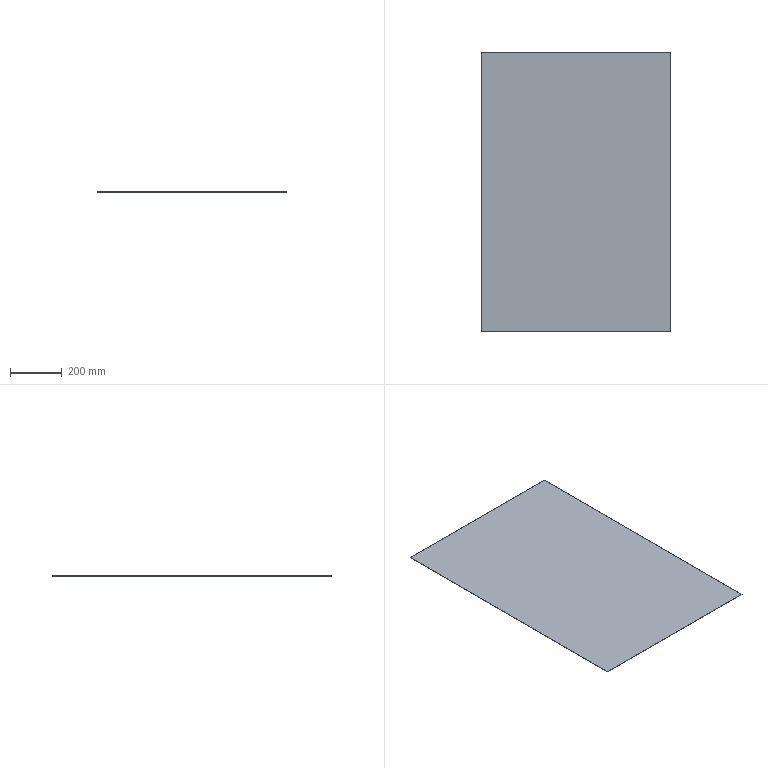Part | STEP file | Guide wheel mechanism revised.sldasm-Part-182 | 1 solid | 6 faces | box 735 x 1085 x 1.2 mm | volume 956970 mm3 | plane 6
STEP:
#1=CARTESIAN_POINT('',(367.5,1897.5,-264.));
#2=VERTEX_POINT('',#1);
#3=CARTESIAN_POINT('',(367.5,812.5,-264.));
#4=VERTEX_POINT('',#3);
#5=CARTESIAN_POINT('',(367.5,1897.5,-264.));
#6=DIRECTION('',(0.,-1.,0.));
#7=VECTOR('',#6,1000.);
#8=LINE('',#5,#7);
#9=EDGE_CURVE('',#2,#4,#8,.T.);
#10=ORIENTED_EDGE('',*,*,#9,.T.);
#11=CARTESIAN_POINT('',(367.5,812.5,-265.2));
#12=VERTEX_POINT('',#11);
#13=CARTESIAN_POINT('',(367.5,812.5,-265.2));
#14=DIRECTION('',(0.,0.,1.));
#15=VECTOR('',#14,1000.);
#16=LINE('',#13,#15);
#17=EDGE_CURVE('',#12,#4,#16,.T.);
#18=ORIENTED_EDGE('',*,*,#17,.F.);
#19=CARTESIAN_POINT('',(367.5,1897.5,-265.2));
#20=VERTEX_POINT('',#19);
#21=CARTESIAN_POINT('',(367.5,1897.5,-265.2));
#22=DIRECTION('',(0.,-1.,0.));
#23=VECTOR('',#22,1000.);
#24=LINE('',#21,#23);
#25=EDGE_CURVE('',#20,#12,#24,.T.);
#26=ORIENTED_EDGE('',*,*,#25,.F.);
#27=CARTESIAN_POINT('',(367.5,1897.5,-265.2));
#28=DIRECTION('',(0.,0.,1.));
#29=VECTOR('',#28,1000.);
#30=LINE('',#27,#29);
#31=EDGE_CURVE('',#20,#2,#30,.T.);
#32=ORIENTED_EDGE('',*,*,#31,.T.);
#33=EDGE_LOOP('',(#10,#18,#26,#32));
#34=FACE_OUTER_BOUND('',#33,.T.);
#35=CARTESIAN_POINT('',(367.5,1897.5,-265.2));
#36=DIRECTION('',(-1.,0.,0.));
#37=DIRECTION('',(0.,-1.,0.));
#38=AXIS2_PLACEMENT_3D('',#35,#36,#37);
#39=PLANE('',#38);
#40=ADVANCED_FACE('',(#34),#39,.F.);
#41=CARTESIAN_POINT('',(-367.5,812.5,-264.));
#42=VERTEX_POINT('',#41);
#43=CARTESIAN_POINT('',(367.5,812.5,-264.));
#44=DIRECTION('',(-1.,0.,0.));
#45=VECTOR('',#44,1000.);
#46=LINE('',#43,#45);
#47=EDGE_CURVE('',#4,#42,#46,.T.);
#48=ORIENTED_EDGE('',*,*,#47,.T.);
#49=CARTESIAN_POINT('',(-367.5,812.5,-265.2));
#50=VERTEX_POINT('',#49);
#51=CARTESIAN_POINT('',(-367.5,812.5,-265.2));
#52=DIRECTION('',(0.,0.,1.));
#53=VECTOR('',#52,1000.);
#54=LINE('',#51,#53);
#55=EDGE_CURVE('',#50,#42,#54,.T.);
#56=ORIENTED_EDGE('',*,*,#55,.F.);
#57=CARTESIAN_POINT('',(367.5,812.5,-265.2));
#58=DIRECTION('',(-1.,0.,0.));
#59=VECTOR('',#58,1000.);
#60=LINE('',#57,#59);
#61=EDGE_CURVE('',#12,#50,#60,.T.);
#62=ORIENTED_EDGE('',*,*,#61,.F.);
#63=ORIENTED_EDGE('',*,*,#17,.T.);
#64=EDGE_LOOP('',(#48,#56,#62,#63));
#65=FACE_OUTER_BOUND('',#64,.T.);
#66=CARTESIAN_POINT('',(367.5,812.5,-265.2));
#67=DIRECTION('',(0.,1.,0.));
#68=DIRECTION('',(0.,0.,1.));
#69=AXIS2_PLACEMENT_3D('',#66,#67,#68);
#70=PLANE('',#69);
#71=ADVANCED_FACE('',(#65),#70,.F.);
#72=CARTESIAN_POINT('',(-367.5,1897.5,-264.));
#73=VERTEX_POINT('',#72);
#74=CARTESIAN_POINT('',(-367.5,1897.5,-264.));
#75=DIRECTION('',(0.,1.,0.));
#76=VECTOR('',#75,1000.);
#77=LINE('',#74,#76);
#78=EDGE_CURVE('',#42,#73,#77,.T.);
#79=ORIENTED_EDGE('',*,*,#78,.T.);
#80=CARTESIAN_POINT('',(-367.5,1897.5,-265.2));
#81=VERTEX_POINT('',#80);
#82=CARTESIAN_POINT('',(-367.5,1897.5,-265.2));
#83=DIRECTION('',(0.,0.,1.));
#84=VECTOR('',#83,1000.);
#85=LINE('',#82,#84);
#86=EDGE_CURVE('',#81,#73,#85,.T.);
#87=ORIENTED_EDGE('',*,*,#86,.F.);
#88=CARTESIAN_POINT('',(-367.5,1897.5,-265.2));
#89=DIRECTION('',(0.,1.,0.));
#90=VECTOR('',#89,1000.);
#91=LINE('',#88,#90);
#92=EDGE_CURVE('',#50,#81,#91,.T.);
#93=ORIENTED_EDGE('',*,*,#92,.F.);
#94=ORIENTED_EDGE('',*,*,#55,.T.);
#95=EDGE_LOOP('',(#79,#87,#93,#94));
#96=FACE_OUTER_BOUND('',#95,.T.);
#97=CARTESIAN_POINT('',(-367.5,1897.5,-265.2));
#98=DIRECTION('',(1.,0.,0.));
#99=DIRECTION('',(0.,1.,0.));
#100=AXIS2_PLACEMENT_3D('',#97,#98,#99);
#101=PLANE('',#100);
#102=ADVANCED_FACE('',(#96),#101,.F.);
#103=CARTESIAN_POINT('',(367.5,1897.5,-264.));
#104=DIRECTION('',(1.,0.,0.));
#105=VECTOR('',#104,1000.);
#106=LINE('',#103,#105);
#107=EDGE_CURVE('',#73,#2,#106,.T.);
#108=ORIENTED_EDGE('',*,*,#107,.T.);
#109=ORIENTED_EDGE('',*,*,#31,.F.);
#110=CARTESIAN_POINT('',(367.5,1897.5,-265.2));
#111=DIRECTION('',(1.,0.,0.));
#112=VECTOR('',#111,1000.);
#113=LINE('',#110,#112);
#114=EDGE_CURVE('',#81,#20,#113,.T.);
#115=ORIENTED_EDGE('',*,*,#114,.F.);
#116=ORIENTED_EDGE('',*,*,#86,.T.);
#117=EDGE_LOOP('',(#108,#109,#115,#116));
#118=FACE_OUTER_BOUND('',#117,.T.);
#119=CARTESIAN_POINT('',(367.5,1897.5,-265.2));
#120=DIRECTION('',(0.,-1.,0.));
#121=DIRECTION('',(0.,0.,-1.));
#122=AXIS2_PLACEMENT_3D('',#119,#120,#121);
#123=PLANE('',#122);
#124=ADVANCED_FACE('',(#118),#123,.F.);
#125=ORIENTED_EDGE('',*,*,#25,.T.);
#126=ORIENTED_EDGE('',*,*,#61,.T.);
#127=ORIENTED_EDGE('',*,*,#92,.T.);
#128=ORIENTED_EDGE('',*,*,#114,.T.);
#129=EDGE_LOOP('',(#125,#126,#127,#128));
#130=FACE_OUTER_BOUND('',#129,.T.);
#131=CARTESIAN_POINT('',(0.,0.,-265.2));
#132=DIRECTION('',(0.,0.,-1.));
#133=DIRECTION('',(-1.,0.,0.));
#134=AXIS2_PLACEMENT_3D('',#131,#132,#133);
#135=PLANE('',#134);
#136=ADVANCED_FACE('',(#130),#135,.T.);
#137=ORIENTED_EDGE('',*,*,#9,.F.);
#138=ORIENTED_EDGE('',*,*,#107,.F.);
#139=ORIENTED_EDGE('',*,*,#78,.F.);
#140=ORIENTED_EDGE('',*,*,#47,.F.);
#141=EDGE_LOOP('',(#137,#138,#139,#140));
#142=FACE_OUTER_BOUND('',#141,.T.);
#143=CARTESIAN_POINT('',(0.,0.,-264.));
#144=DIRECTION('',(0.,0.,-1.));
#145=DIRECTION('',(-1.,0.,0.));
#146=AXIS2_PLACEMENT_3D('',#143,#144,#145);
#147=PLANE('',#146);
#148=ADVANCED_FACE('',(#142),#147,.F.);
#149=CLOSED_SHELL('',(#40,#71,#102,#124,#136,#148));
#150=MANIFOLD_SOLID_BREP('',#149);
#151=CARTESIAN_POINT('',(0.,0.,0.));
#152=DIRECTION('',(0.,0.,1.));
#153=DIRECTION('',(1.,0.,0.));
#154=AXIS2_PLACEMENT_3D('',#151,#152,#153);
#155=(LENGTH_UNIT()NAMED_UNIT(*)SI_UNIT(.MILLI.,.METRE.));
#156=UNCERTAINTY_MEASURE_WITH_UNIT(LENGTH_MEASURE(0.00001),#155,'','');
#157=(NAMED_UNIT(*)PLANE_ANGLE_UNIT()SI_UNIT($,.RADIAN.));
#158=(NAMED_UNIT(*)SI_UNIT($,.STERADIAN.)SOLID_ANGLE_UNIT());
#159=(GEOMETRIC_REPRESENTATION_CONTEXT(3)GLOBAL_UNCERTAINTY_ASSIGNED_CONTEXT((#156))GLOBAL_UNIT_ASSIGNED_CONTEXT((#155,#157,#158))REPRESENTATION_CONTEXT('',''));
#160=ADVANCED_BREP_SHAPE_REPRESENTATION('',(#150,#154),#159);